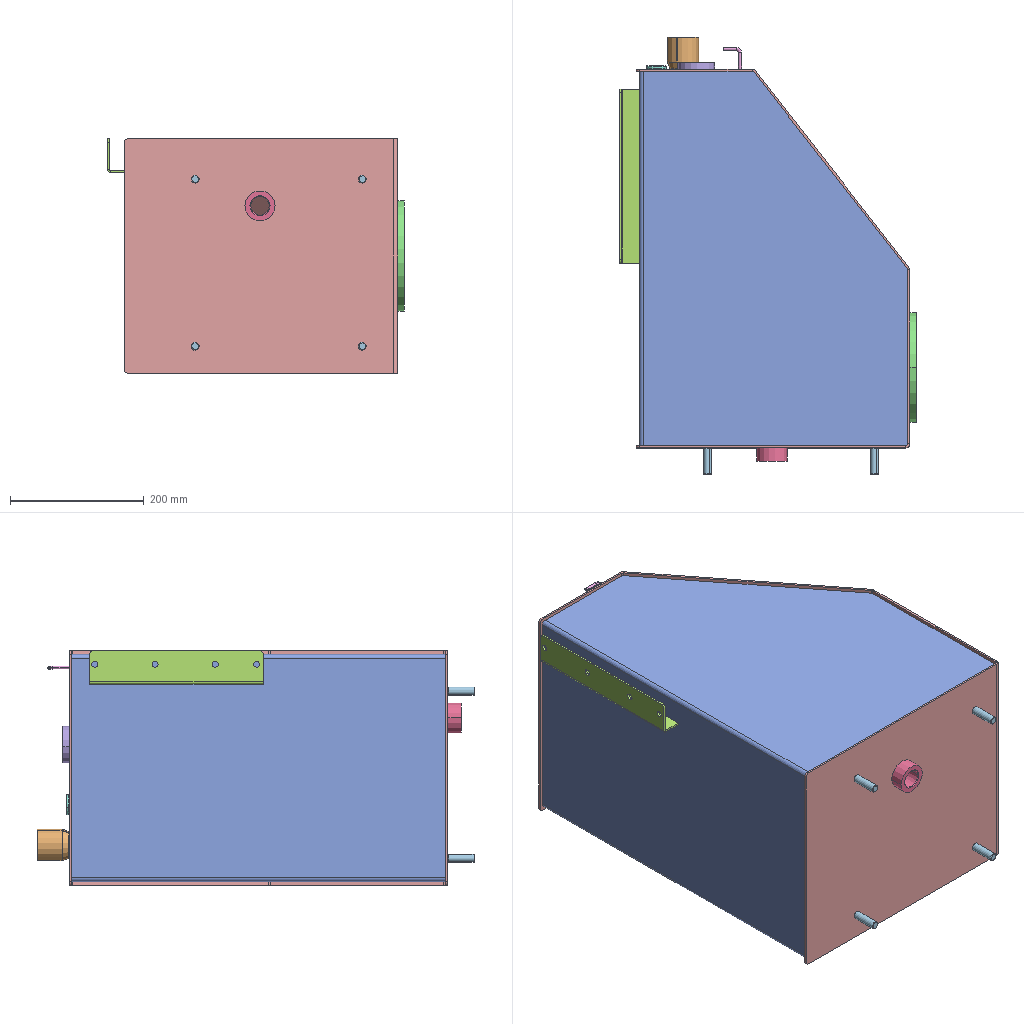Assembly | SolidWorks | 10 different items | 13 placed | box 444 x 654 x 350 mm
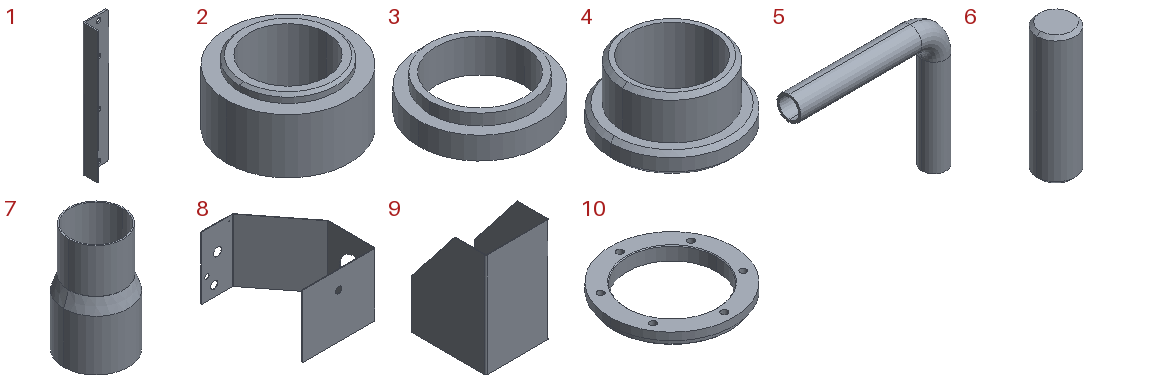Parts list (item | quantity | size | volume | features):
1 | x1 | 50 x 30 x 260 mm | 58427 mm3 | features FlatPattern 1, ICE 1, SMBaseFlange 1, SheetMetal 1
2 | x1 | 45 x 45 x 23 mm | 20434 mm3 | features Chamfer 1, Extrusion 1, ICE 1
3 | x1 | 55 x 55 x 15 mm | 13492 mm3 | features Extrusion 1, ICE 1
4 | x1 | 30 x 30 x 15 mm | 3311 mm3 | features Chamfer 1, Extrusion 1, ICE 1
5 | x1 | 32.5 x 5 x 27.5 mm | 373.603 mm3 | features Sweep 1
6 | x4 | 11.85 x 11.85 x 40 mm | 4376 mm3 | features Chamfer 1, Extrusion 1
7 | x1 | 47 x 47 x 79 mm | 10172 mm3 | features 3DProfileFeature 2, ICE 2, NetBlend 1, NetBlendCut 1
8 | x1 | 409 x 566 x 350 mm | 1214329 mm3 | features ICE 4, FlatPattern 1, SMBaseFlange 1, SheetMetal 1
9 | x1 | 340 x 401 x 560 mm | 1696570 mm3 | features FlatPattern 1, ICE 1, SMBaseFlange 1, SheetMetal 1
10 | x1 | 165 x 165 x 18 mm | 159935 mm3 | features ICE 2, Chamfer 1, Extrusion 1
Mates (type | each side: item.copy, entity, surface, feature):
DistanceDim | 9.1 face plane Base-Flange1 | 8.1 face plane Base-Flange1
Coincident | 8.1 face plane Base-Flange1 | 9.1 face plane Base-Flange1 | 2 times
Coincident | 9.1 face plane Base-Flange1 | 1.1 face plane Base-Flange1
DistanceDim | 1.1 face plane Base-Flange1 | 8.1 face plane Base-Flange1
Coincident | 8.1 face plane Base-Flange1 | 1.1 face plane Base-Flange1
Concentric | 8.1 edge | 4.1 edge
Coincident | 8.1 face plane Base-Flange1 | 4.1 edge
Concentric | 8.1 edge | 5.1 edge
Coincident | 8.1 face plane Base-Flange1 | 5.1 face plane Sweep1
Parallel | 8.1 face plane Base-Flange1 | 5.1 face plane Sweep1
Concentric | 8.1 edge | 7.1 edge
DistanceDim | 7.1 face plane Boss-Extrude1 | 8.1 face plane Base-Flange1
Concentric | 8.1 edge | 3.1 edge
Coincident | 8.1 face plane Base-Flange1 | 3.1 face plane Boss-Extrude1
Concentric | 8.1 edge | 10.1 edge
Coincident | 8.1 face plane Base-Flange1 | 10.1 face plane Boss-Extrude1
Coincident | 8.1 face plane Base-Flange1 | 2.1 face plane Boss-Extrude1
Concentric | 8.1 edge | 2.1 face cone Chamfer1
Coincident | 6.1 face plane Boss-Extrude1 | 6.2 face plane Boss-Extrude1
Coincident | 6.1 face plane Boss-Extrude1 | 6.3 face plane Boss-Extrude1
Coincident | 6.4 face plane Boss-Extrude1 | 6.3 face plane Boss-Extrude1
Coincident | 8.1 face plane Base-Flange1 | 6.2 face plane Boss-Extrude1
Concentric | 6.2 edge | assembly select_type:10
Concentric | 6.1 edge | assembly select_type:10
Concentric | 6.3 edge | assembly select_type:10
Concentric | 6.4 edge | assembly select_type:10